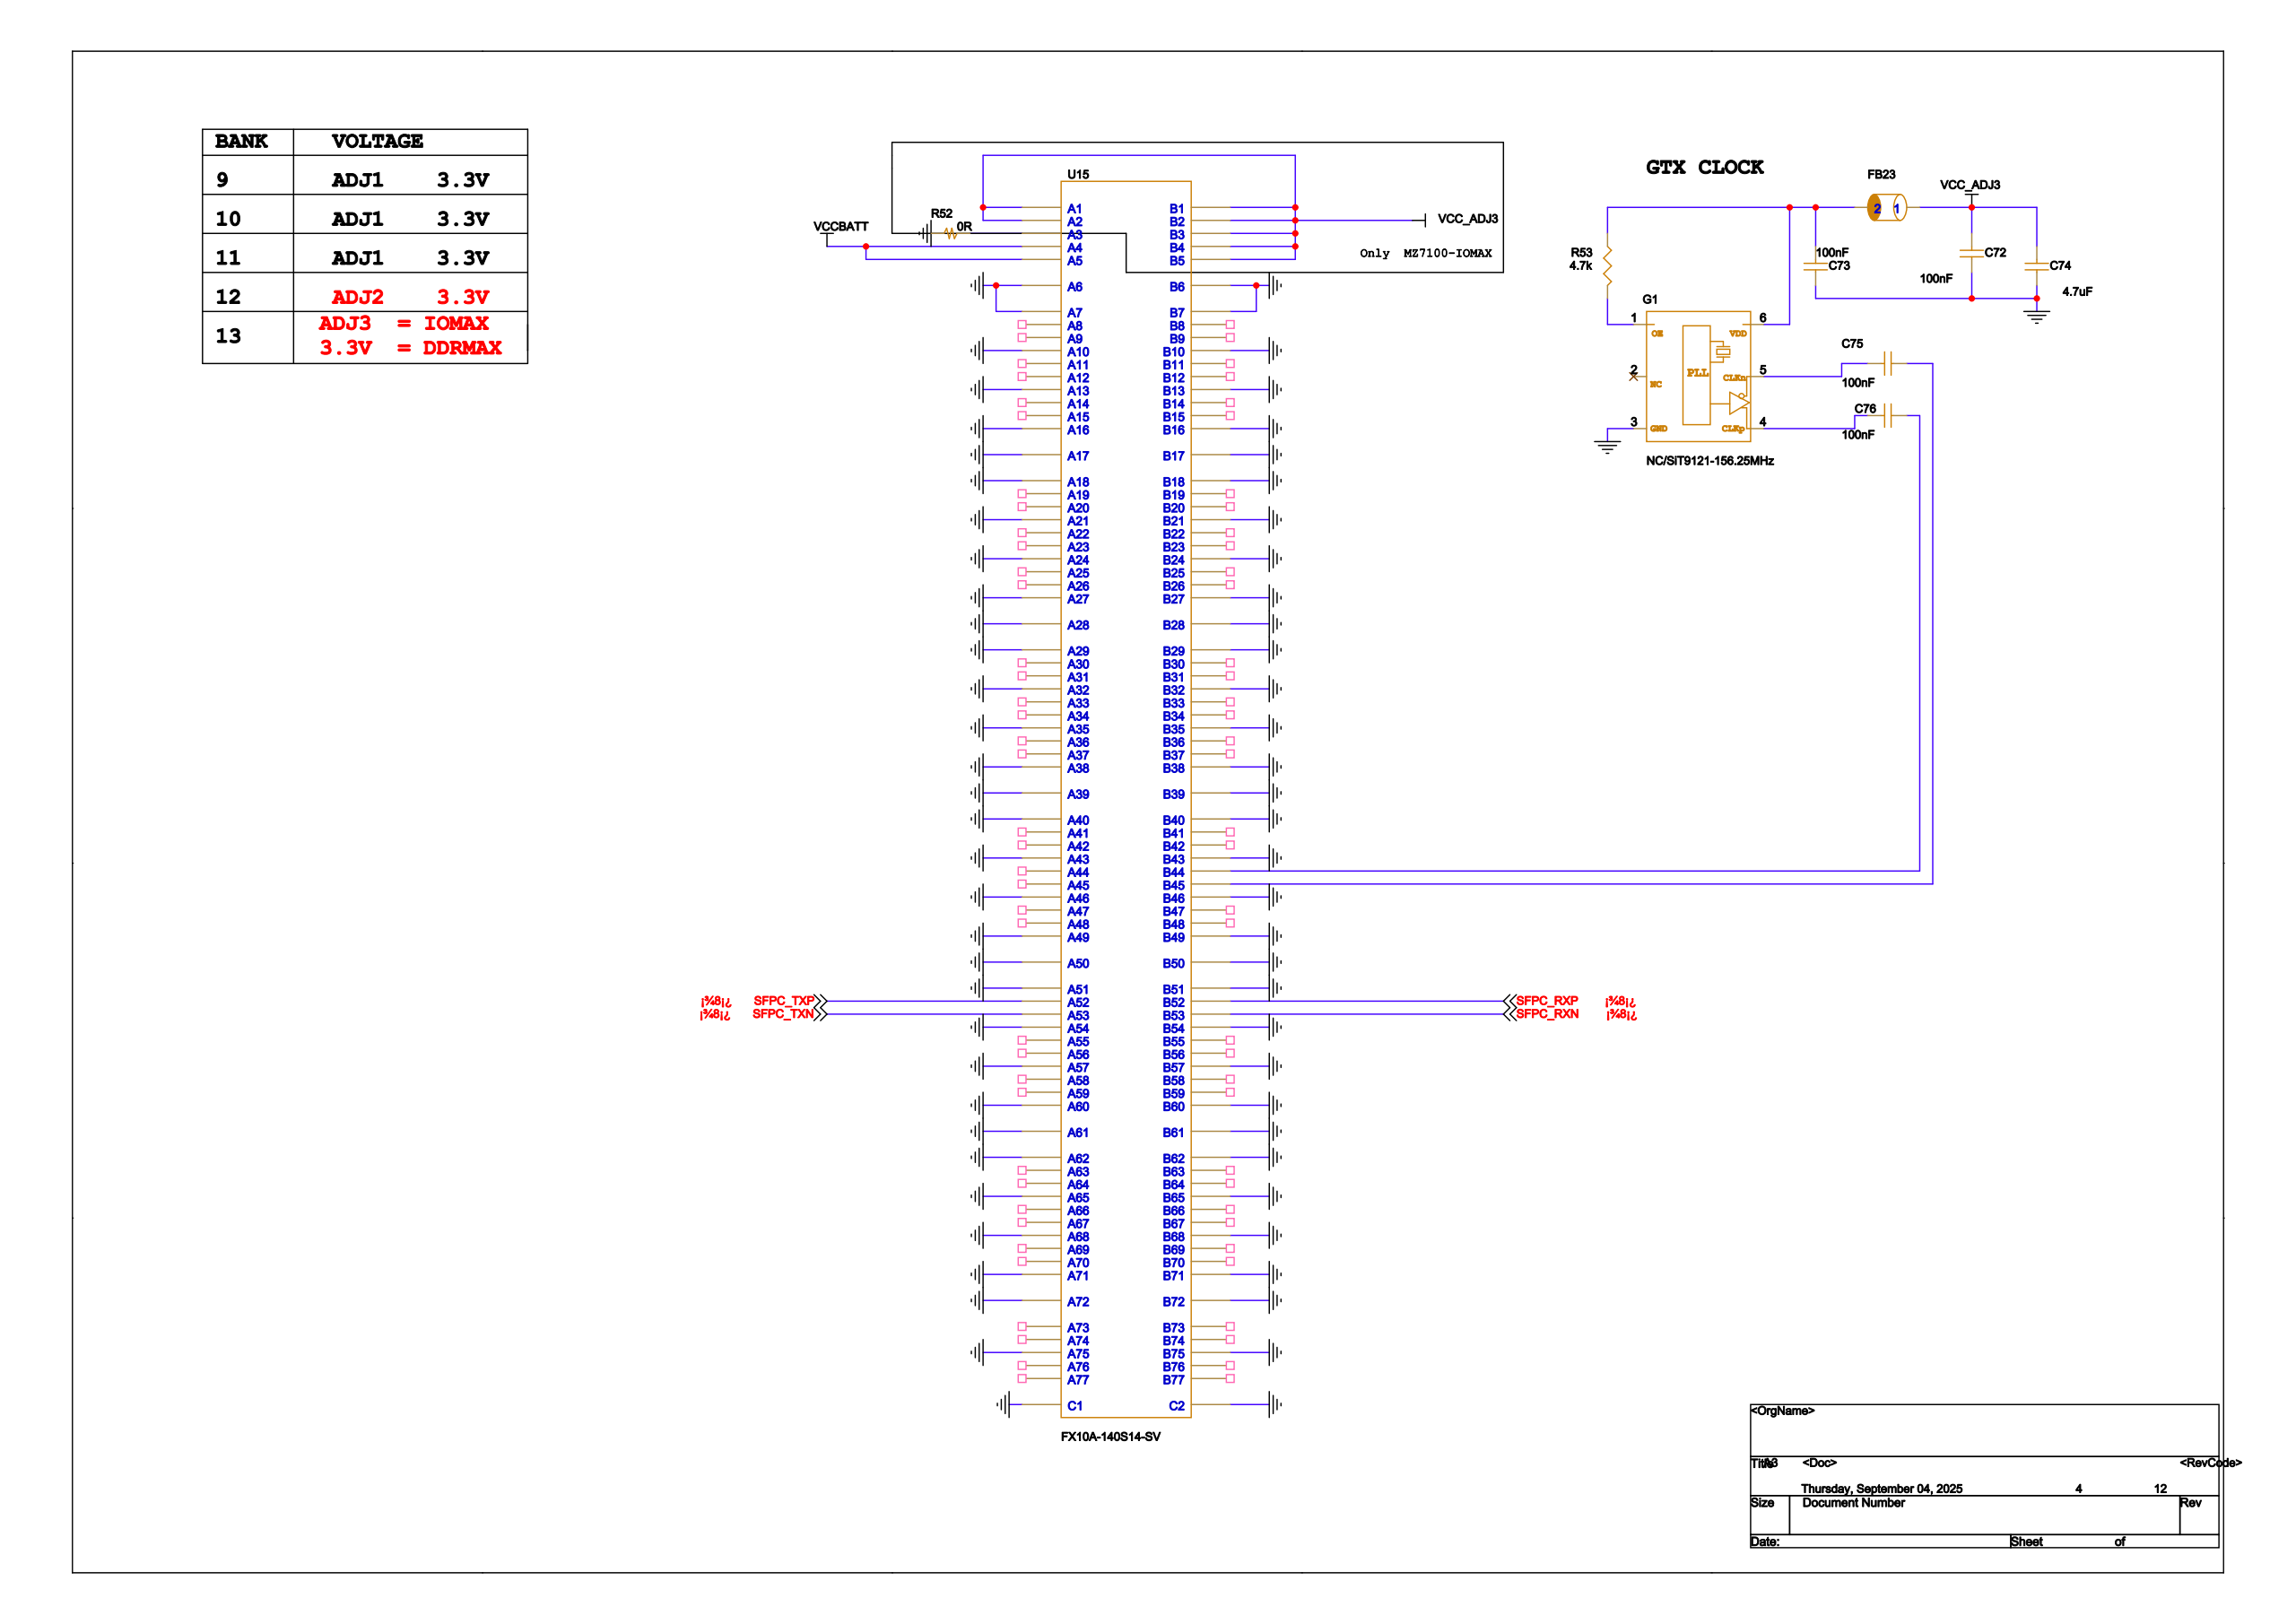Circuit board | Cadence Allegro | 528 parts | 530 nets | one sheet of the schematic
Parts on this sheet (reference | value | footprint):
C72 | 100nF | C0402
C73 | 100nF | C0402
C74 | 4.7uF | C0603
C75 | 100nF | C0402
C76 | 100nF | C0402
FB23 | BLM18PG121SN1 | 0603
G1 | NC/SiT9121-156.25MHz | OSC6-3225
R52 | 0R | R0402
R53 | 4.7k | R0402
U15 | FX10A-140S14-SV | FX10A-140S14-SV
Nets of these parts (net: part-pin ...):
GND: C72-1 C73-1 C74-1 G1-3 R52-1 U15-C1 U15-C2
VCC_ADJ3: C72-2 C74-2 FB23-1
N17502430: C73-2 FB23-2 G1-6 R53-1
N17502524: C75-1
N17502522: C75-2 G1-5
N17502542: C76-1
N17502540: C76-2 G1-4
N17502488: G1-1 R53-2
N19535138: R52-2